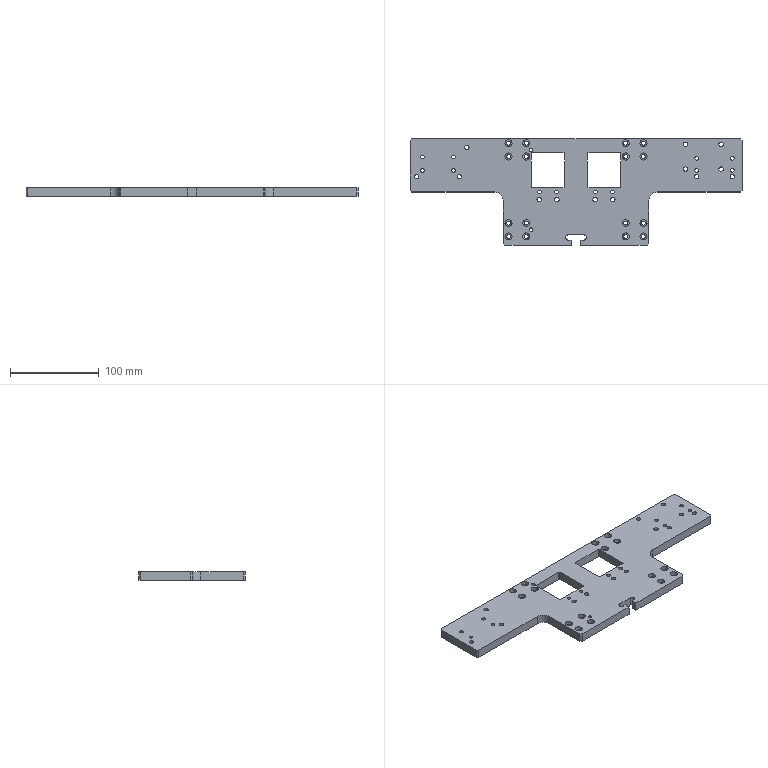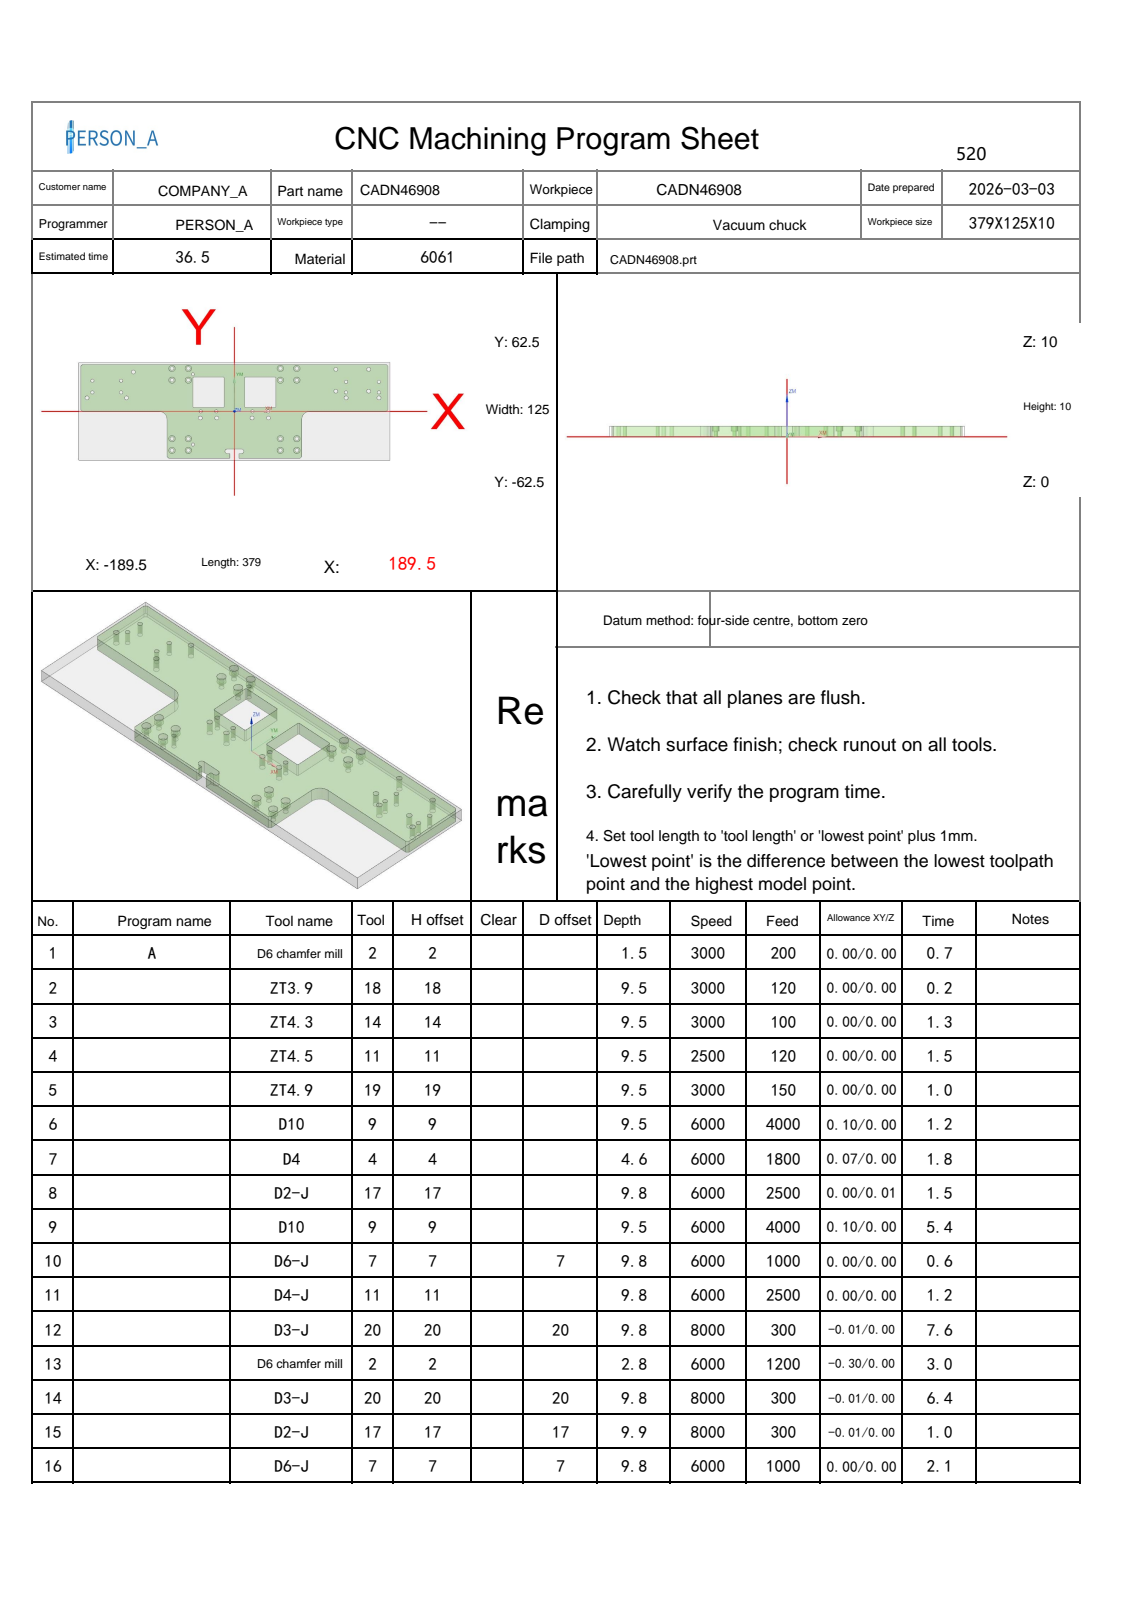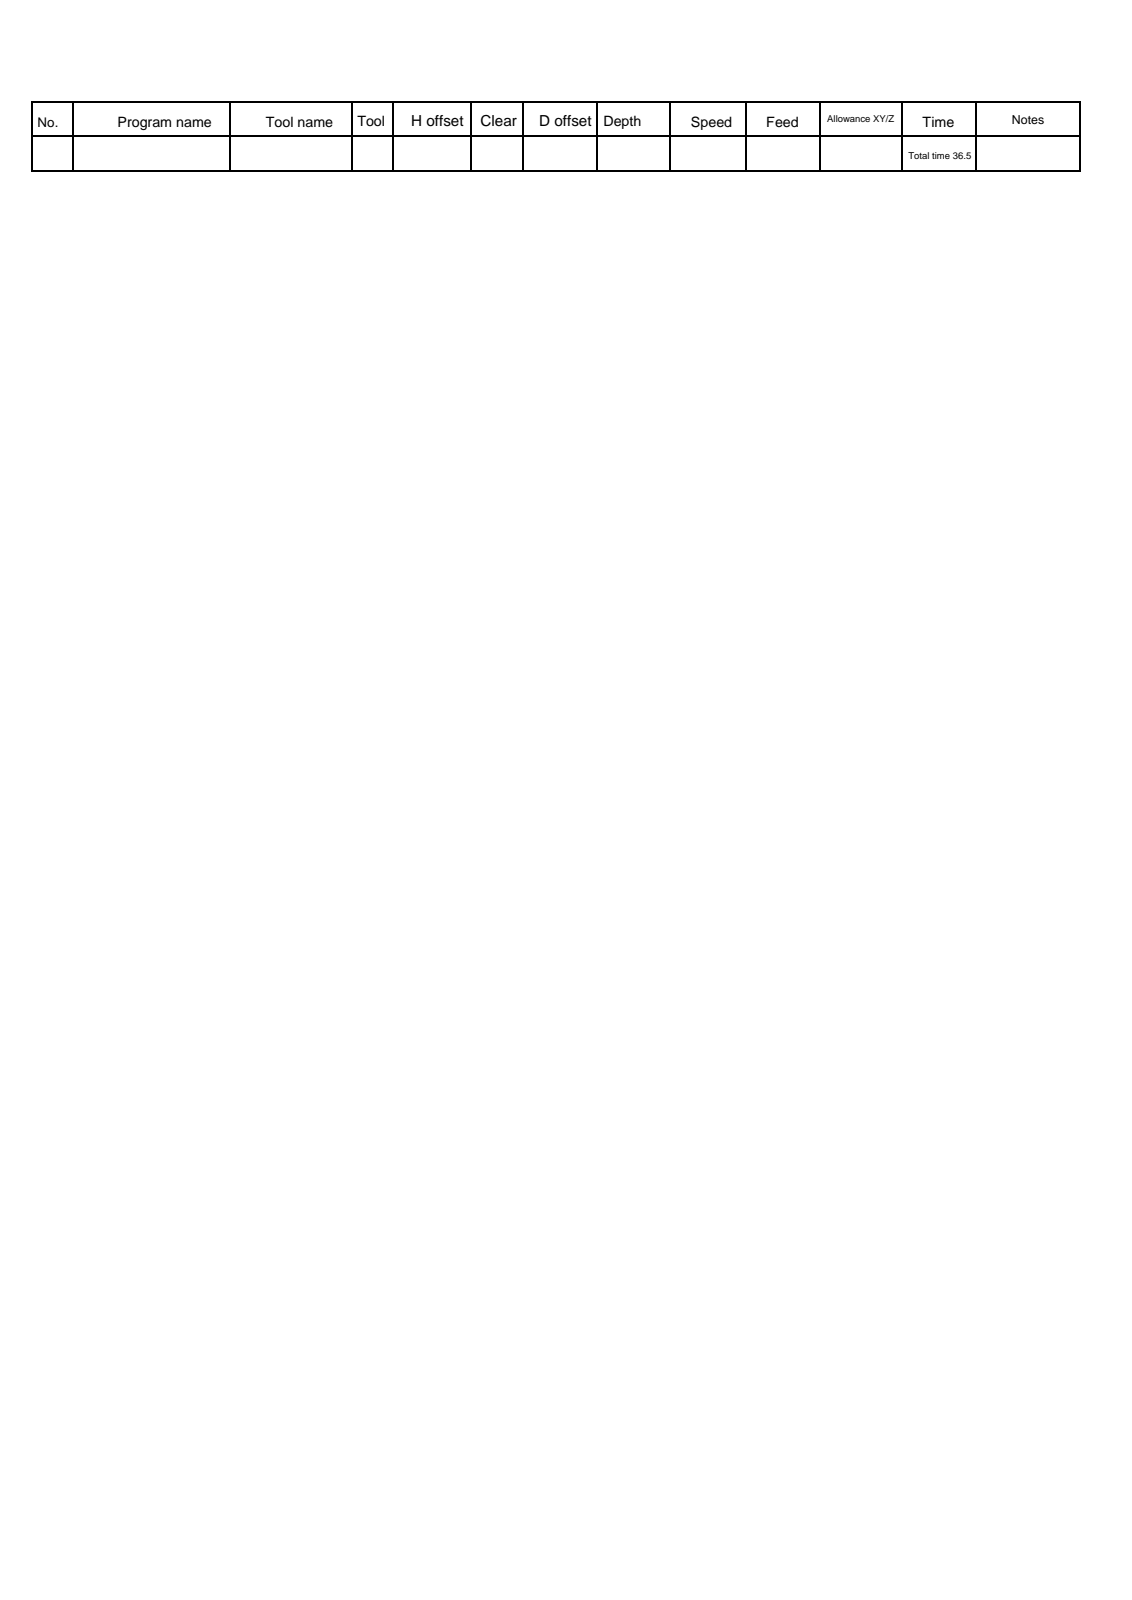NC program | NX | posted by the shop | part box 374 x 120 x 10 mm
Lines 1 to 769 of 15301:
%
O0001
(Machine time: 39.34 MIN)
(===Total Tool:10===)
(T2=D6 chamfer mill   D=6.   R=0.   D-  H02 Z=7.2   )
(T18=ZT3.9  D=3.9  DR_a=120 D-  H18 Z=0.5   )
(T14=ZT4.3  D=4.3  DR_a=118 D-  H14 Z=0.5   )
(T11=ZT4.5  D=4.5  DR_a=118 D-  H11 Z=0.2   )
(T19=ZT4.9  D=4.9  DR_a=120 D-  H19 Z=0.5   )
(T9=D10     D=10.  R=0.   D-  H09 Z=0.5   )
(T4=D4      D=4.   R=0.   D-  H04 Z=5.4   )
(T17=D2-J   D=2.   R=0.   D-  H17 Z=0.15  )
(T7=D6-J    D=6.   R=0.   D7  H07 Z=0.2   )
(T20=D3-J   D=3.   R=0.   D20 H20 Z=0.15  )
G80 G90 G17 G49 G40
G91 G28 Z0
M01
N1 T02 M06
(D6 chamfer mill  D=6. R=0. H=02 ce=0.00 di=0.00)
G00 G90 G54 X176. Y17.3 M03 S3000
G43 H02 Z40.
M08
G98 G82 X176. Y17.3 Z8.5 R11. F200.
X163.5 Y25.8
Y53.8
X123.5
Y25.8
X136. Y17.3
X41.5 Y-8.5
X21.5
X-21.5
X-41.5
X-122.971 Y50.4
X-131.471 Y17.3
X-179.471
G80
G00 Z40.
G00 G90 X-172.971 Y39.3 M03 S3000
Z40.
G98 G81 X-172.971 Y39.3 Z8.5 R11. F200.
Y24.3
X-137.971
Y39.3
X-76. Y40.
Y55.
X-56.
X-50.5 Y47.5
X-56. Y40.
X-76. Y-35.
Y-50.
X-56.
X-50.5 Y-42.5
X-56. Y-35.
X-41. Y0.0
X-22.
X22.
X41.
X56. Y-35.
Y-50.
X76.
Y-35.
X56. Y40.
Y55.
X76.
Y40.
X136. Y37.8
Y24.3
X176.
Y37.8
G80
G00 Z40.
G91 G28 Z0.0
M05
M09
G91 G28 Z0.0
M01
N2 T18 M06
(ZT3.9 D=3.9 DR_a=120 H=18)
G00 G90 G54 X-50.5 Y-42.5 M03 S3000
G43 H18 Z40.
M08
G98 G83 X-50.5 Y-42.5 Z.5 R11. F120. Q2.
Y47.5
G80
G00 Z40.
G91 G28 Z0.0
M05
M09
G91 G28 Z0.0
M01
N3 T14 M06
(ZT4.3 D=4.3 DR_a=118 H=14)
G00 G90 G54 X-172.971 Y24.3 M03 S3000
G43 H14 Z40.
M08
G98 G83 X-172.971 Y24.3 Z.5 R11. F100. Q1.5
Y39.3
X-137.971
Y24.3
X-41. Y0.0
X-22.
X22.
X41.
X136. Y24.3
Y37.8
X176.
Y24.3
G80
G00 Z40.
G91 G28 Z0.0
M05
M09
G91 G28 Z0.0
M01
N4 T11 M06
(ZT4.5 D=4.5 DR_a=118 H=11)
G00 G90 G54 X56. Y-35. M03 S2500
G43 H11 Z40.
M08
G98 G83 X56. Y-35. Z.5 R11. F120. Q3.
Y-50.
X76.
Y-35.
Y40.
Y55.
X56.
Y40.
X-56.
Y55.
X-76.
Y40.
Y-35.
Y-50.
X-56.
Y-35.
G80
G00 Z40.
G91 G28 Z0.0
M05
M09
G91 G28 Z0.0
M01
N5 T19 M06
(ZT4.9 D=4.9 DR_a=120 H=19)
G00 G90 G54 X176. Y17.3 M03 S3000
G43 H19 Z40.
M08
G98 G83 X176. Y17.3 Z.5 R11. F150. Q3.
X163.5 Y25.8
Y53.8
X123.5
Y25.8
X136. Y17.3
X41.5 Y-8.5
X21.5
X-21.5
X-41.5
X-122.971 Y50.4
X-131.471 Y17.3
X-179.471
G80
G00 Z40.
G91 G28 Z0.0
M05
M09
G91 G28 Z0.0
M01
N6 T09 M06
(D10  D=10. R=0. H=09 ce=0.10 di=0.00)
G00 G90 G54 X-31.5 Y38.9 M03 S6000
G43 H09 Z40.
M08
Z10.5
G01 X-45.4 Z10.439 F4000.
Y10.1 Z10.311
X-17.6 Z10.189
Y38.9 Z10.061
X-45.4 Z9.939
Y10.1 Z9.811
X-17.6 Z9.689
Y38.9 Z9.561
X-45.4 Z9.439
Y10.1 Z9.311
X-17.6 Z9.189
Y38.9 Z9.061
X-45.4 Z8.939
Y10.1 Z8.811
X-17.6 Z8.689
Y38.9 Z8.561
X-45.4 Z8.439
Y10.1 Z8.311
X-17.6 Z8.189
Y38.9 Z8.061
X-45.4 Z7.939
Y10.1 Z7.811
X-17.6 Z7.689
Y38.9 Z7.561
X-45.4 Z7.439
Y10.1 Z7.311
X-17.6 Z7.189
Y38.9 Z7.061
X-45.4 Z6.939
Y10.1 Z6.811
X-17.6 Z6.689
Y38.9 Z6.561
X-45.4 Z6.439
Y10.1 Z6.311
X-17.6 Z6.189
Y38.9 Z6.061
X-45.4 Z5.939
Y10.1 Z5.811
X-17.6 Z5.689
Y38.9 Z5.561
X-45.4 Z5.439
Y10.1 Z5.311
X-17.6 Z5.189
Y38.9 Z5.061
X-45.4 Z4.939
Y10.1 Z4.811
X-17.6 Z4.689
Y38.9 Z4.561
X-45.4 Z4.439
Y10.1 Z4.311
X-17.6 Z4.189
Y38.9 Z4.061
X-45.4 Z3.939
Y10.1 Z3.811
X-17.6 Z3.689
Y38.9 Z3.561
X-45.4 Z3.439
Y10.1 Z3.311
X-17.6 Z3.189
Y38.9 Z3.061
X-45.4 Z2.939
Y10.1 Z2.811
X-17.6 Z2.689
Y38.9 Z2.561
X-45.4 Z2.439
Y10.1 Z2.311
X-17.6 Z2.189
Y38.9 Z2.061
X-45.4 Z1.939
Y10.1 Z1.811
X-17.6 Z1.689
Y38.9 Z1.561
X-45.4 Z1.439
Y10.1 Z1.311
X-17.6 Z1.189
Y38.9 Z1.061
X-45.4 Z.939
Y10.1 Z.811
X-17.6 Z.689
Y38.9 Z.561
X-31.5 Z.5
X-45.4
Y10.1
X-17.6
Y38.9
X-31.5
X-32.
Z1.5
G00 Z40.
X31.5
Z10.5
G01 X17.6 Z10.439
Y10.1 Z10.311
X45.4 Z10.189
Y38.9 Z10.061
X17.6 Z9.939
Y10.1 Z9.811
X45.4 Z9.689
Y38.9 Z9.561
X17.6 Z9.439
Y10.1 Z9.311
X45.4 Z9.189
Y38.9 Z9.061
X17.6 Z8.939
Y10.1 Z8.811
X45.4 Z8.689
Y38.9 Z8.561
X17.6 Z8.439
Y10.1 Z8.311
X45.4 Z8.189
Y38.9 Z8.061
X17.6 Z7.939
Y10.1 Z7.811
X45.4 Z7.689
Y38.9 Z7.561
X17.6 Z7.439
Y10.1 Z7.311
X45.4 Z7.189
Y38.9 Z7.061
X17.6 Z6.939
Y10.1 Z6.811
X45.4 Z6.689
Y38.9 Z6.561
X17.6 Z6.439
Y10.1 Z6.311
X45.4 Z6.189
Y38.9 Z6.061
X17.6 Z5.939
Y10.1 Z5.811
X45.4 Z5.689
Y38.9 Z5.561
X17.6 Z5.439
Y10.1 Z5.311
X45.4 Z5.189
Y38.9 Z5.061
X17.6 Z4.939
Y10.1 Z4.811
X45.4 Z4.689
Y38.9 Z4.561
X17.6 Z4.439
Y10.1 Z4.311
X45.4 Z4.189
Y38.9 Z4.061
X17.6 Z3.939
Y10.1 Z3.811
X45.4 Z3.689
Y38.9 Z3.561
X17.6 Z3.439
Y10.1 Z3.311
X45.4 Z3.189
Y38.9 Z3.061
X17.6 Z2.939
Y10.1 Z2.811
X45.4 Z2.689
Y38.9 Z2.561
X17.6 Z2.439
Y10.1 Z2.311
X45.4 Z2.189
Y38.9 Z2.061
X17.6 Z1.939
Y10.1 Z1.811
X45.4 Z1.689
Y38.9 Z1.561
X17.6 Z1.439
Y10.1 Z1.311
X45.4 Z1.189
Y38.9 Z1.061
X17.6 Z.939
Y10.1 Z.811
X45.4 Z.689
Y38.9 Z.561
X31.5 Z.5
X17.6
Y10.1
X45.4
Y38.9
X31.5
X31.
Z1.5
G00 Z40.
G91 G28 Z0.0
M05
M09
G91 G28 Z0.0
M01
N7 T04 M06
(D4  D=4. R=0. H=04 ce=0.07 di=0.00)
G00 G90 G54 X-76. Y55. M03 S6000
G43 H04 Z40.
M08
Z10.3
G03 X-75.035 Y54.035 I.965 J0.0 F1800.
X-74.07 Y55. I0.0 J.965
X-74.07 Y55. Z9.95 I-1.93 J0.0
X-74.07 Y55. Z9.6 I-1.93 J0.0
X-74.07 Y55. Z9.25 I-1.93 J0.0
X-74.07 Y55. Z8.9 I-1.93 J0.0
X-74.07 Y55. Z8.55 I-1.93 J0.0
X-74.07 Y55. Z8.2 I-1.93 J0.0
X-74.07 Y55. Z7.85 I-1.93 J0.0
X-74.07 Y55. Z7.5 I-1.93 J0.0
X-74.07 Y55. Z7.15 I-1.93 J0.0
X-74.07 Y55. Z6.8 I-1.93 J0.0
X-74.07 Y55. Z6.45 I-1.93 J0.0
X-74.07 Y55. Z6.1 I-1.93 J0.0
X-74.07 Y55. Z5.75 I-1.93 J0.0
X-74.07 Y55. Z5.4 I-1.93 J0.0
X-76. Y56.93 I-1.93 J0.0
X-77.93 Y55. I0.0 J-1.93
X-76. Y53.07 I1.93 J0.0
X-74.07 Y55. I0.0 J1.93
X-75.035 Y55.965 I-.965 J0.0
X-76. Y55. I0.0 J-.965
G00 Z40.
X-56.
Z10.3
G03 X-55.035 Y54.035 I.965 J0.0
X-54.07 Y55. I0.0 J.965
X-54.07 Y55. Z9.95 I-1.93 J0.0
X-54.07 Y55. Z9.6 I-1.93 J0.0
X-54.07 Y55. Z9.25 I-1.93 J0.0
X-54.07 Y55. Z8.9 I-1.93 J0.0
X-54.07 Y55. Z8.55 I-1.93 J0.0
X-54.07 Y55. Z8.2 I-1.93 J0.0
X-54.07 Y55. Z7.85 I-1.93 J0.0
X-54.07 Y55. Z7.5 I-1.93 J0.0
X-54.07 Y55. Z7.15 I-1.93 J0.0
X-54.07 Y55. Z6.8 I-1.93 J0.0
X-54.07 Y55. Z6.45 I-1.93 J0.0
X-54.07 Y55. Z6.1 I-1.93 J0.0
X-54.07 Y55. Z5.75 I-1.93 J0.0
X-54.07 Y55. Z5.4 I-1.93 J0.0
X-56. Y56.93 I-1.93 J0.0
X-57.93 Y55. I0.0 J-1.93
X-56. Y53.07 I1.93 J0.0
X-54.07 Y55. I0.0 J1.93
X-55.035 Y55.965 I-.965 J0.0
X-56. Y55. I0.0 J-.965
G00 Z40.
Y40.
Z10.3
G03 X-55.035 Y39.035 I.965 J0.0
X-54.07 Y40. I0.0 J.965
X-54.07 Y40. Z9.95 I-1.93 J0.0
X-54.07 Y40. Z9.6 I-1.93 J0.0
X-54.07 Y40. Z9.25 I-1.93 J0.0
X-54.07 Y40. Z8.9 I-1.93 J0.0
X-54.07 Y40. Z8.55 I-1.93 J0.0
X-54.07 Y40. Z8.2 I-1.93 J0.0
X-54.07 Y40. Z7.85 I-1.93 J0.0
X-54.07 Y40. Z7.5 I-1.93 J0.0
X-54.07 Y40. Z7.15 I-1.93 J0.0
X-54.07 Y40. Z6.8 I-1.93 J0.0
X-54.07 Y40. Z6.45 I-1.93 J0.0
X-54.07 Y40. Z6.1 I-1.93 J0.0
X-54.07 Y40. Z5.75 I-1.93 J0.0
X-54.07 Y40. Z5.4 I-1.93 J0.0
X-56. Y41.93 I-1.93 J0.0
X-57.93 Y40. I0.0 J-1.93
X-56. Y38.07 I1.93 J0.0
X-54.07 Y40. I0.0 J1.93
X-55.035 Y40.965 I-.965 J0.0
X-56. Y40. I0.0 J-.965
G00 Z40.
X-76.
Z10.3
G03 X-75.035 Y39.035 I.965 J0.0
X-74.07 Y40. I0.0 J.965
X-74.07 Y40. Z9.95 I-1.93 J0.0
X-74.07 Y40. Z9.6 I-1.93 J0.0
X-74.07 Y40. Z9.25 I-1.93 J0.0
X-74.07 Y40. Z8.9 I-1.93 J0.0
X-74.07 Y40. Z8.55 I-1.93 J0.0
X-74.07 Y40. Z8.2 I-1.93 J0.0
X-74.07 Y40. Z7.85 I-1.93 J0.0
X-74.07 Y40. Z7.5 I-1.93 J0.0
X-74.07 Y40. Z7.15 I-1.93 J0.0
X-74.07 Y40. Z6.8 I-1.93 J0.0
X-74.07 Y40. Z6.45 I-1.93 J0.0
X-74.07 Y40. Z6.1 I-1.93 J0.0
X-74.07 Y40. Z5.75 I-1.93 J0.0
X-74.07 Y40. Z5.4 I-1.93 J0.0
X-76. Y41.93 I-1.93 J0.0
X-77.93 Y40. I0.0 J-1.93
X-76. Y38.07 I1.93 J0.0
X-74.07 Y40. I0.0 J1.93
X-75.035 Y40.965 I-.965 J0.0
X-76. Y40. I0.0 J-.965
G00 Z40.
Y-35.
Z10.3
G03 X-75.035 Y-35.965 I.965 J0.0
X-74.07 Y-35. I0.0 J.965
X-74.07 Y-35. Z9.95 I-1.93 J0.0
X-74.07 Y-35. Z9.6 I-1.93 J0.0
X-74.07 Y-35. Z9.25 I-1.93 J0.0
X-74.07 Y-35. Z8.9 I-1.93 J0.0
X-74.07 Y-35. Z8.55 I-1.93 J0.0
X-74.07 Y-35. Z8.2 I-1.93 J0.0
X-74.07 Y-35. Z7.85 I-1.93 J0.0
X-74.07 Y-35. Z7.5 I-1.93 J0.0
X-74.07 Y-35. Z7.15 I-1.93 J0.0
X-74.07 Y-35. Z6.8 I-1.93 J0.0
X-74.07 Y-35. Z6.45 I-1.93 J0.0
X-74.07 Y-35. Z6.1 I-1.93 J0.0
X-74.07 Y-35. Z5.75 I-1.93 J0.0
X-74.07 Y-35. Z5.4 I-1.93 J0.0
X-76. Y-33.07 I-1.93 J0.0
X-77.93 Y-35. I0.0 J-1.93
X-76. Y-36.93 I1.93 J0.0
X-74.07 Y-35. I0.0 J1.93
X-75.035 Y-34.035 I-.965 J0.0
X-76. Y-35. I0.0 J-.965
G00 Z40.
Y-50.
Z10.3
G03 X-75.035 Y-50.965 I.965 J0.0
X-74.07 Y-50. I0.0 J.965
X-74.07 Y-50. Z9.95 I-1.93 J0.0
X-74.07 Y-50. Z9.6 I-1.93 J0.0
X-74.07 Y-50. Z9.25 I-1.93 J0.0
X-74.07 Y-50. Z8.9 I-1.93 J0.0
X-74.07 Y-50. Z8.55 I-1.93 J0.0
X-74.07 Y-50. Z8.2 I-1.93 J0.0
X-74.07 Y-50. Z7.85 I-1.93 J0.0
X-74.07 Y-50. Z7.5 I-1.93 J0.0
X-74.07 Y-50. Z7.15 I-1.93 J0.0
X-74.07 Y-50. Z6.8 I-1.93 J0.0
X-74.07 Y-50. Z6.45 I-1.93 J0.0
X-74.07 Y-50. Z6.1 I-1.93 J0.0
X-74.07 Y-50. Z5.75 I-1.93 J0.0
X-74.07 Y-50. Z5.4 I-1.93 J0.0
X-76. Y-48.07 I-1.93 J0.0
X-77.93 Y-50. I0.0 J-1.93
X-76. Y-51.93 I1.93 J0.0
X-74.07 Y-50. I0.0 J1.93
X-75.035 Y-49.035 I-.965 J0.0
X-76. Y-50. I0.0 J-.965
G00 Z40.
X-56.
Z10.3
G03 X-55.035 Y-50.965 I.965 J0.0
X-54.07 Y-50. I0.0 J.965
X-54.07 Y-50. Z9.95 I-1.93 J0.0
X-54.07 Y-50. Z9.6 I-1.93 J0.0
X-54.07 Y-50. Z9.25 I-1.93 J0.0
X-54.07 Y-50. Z8.9 I-1.93 J0.0
X-54.07 Y-50. Z8.55 I-1.93 J0.0
X-54.07 Y-50. Z8.2 I-1.93 J0.0
X-54.07 Y-50. Z7.85 I-1.93 J0.0
X-54.07 Y-50. Z7.5 I-1.93 J0.0
X-54.07 Y-50. Z7.15 I-1.93 J0.0
X-54.07 Y-50. Z6.8 I-1.93 J0.0
X-54.07 Y-50. Z6.45 I-1.93 J0.0
X-54.07 Y-50. Z6.1 I-1.93 J0.0
X-54.07 Y-50. Z5.75 I-1.93 J0.0
X-54.07 Y-50. Z5.4 I-1.93 J0.0
X-56. Y-48.07 I-1.93 J0.0
X-57.93 Y-50. I0.0 J-1.93
X-56. Y-51.93 I1.93 J0.0
X-54.07 Y-50. I0.0 J1.93
X-55.035 Y-49.035 I-.965 J0.0
X-56. Y-50. I0.0 J-.965
G00 Z40.
Y-35.
Z10.3
G03 X-55.035 Y-35.965 I.965 J0.0
X-54.07 Y-35. I0.0 J.965
X-54.07 Y-35. Z9.95 I-1.93 J0.0
X-54.07 Y-35. Z9.6 I-1.93 J0.0
X-54.07 Y-35. Z9.25 I-1.93 J0.0
X-54.07 Y-35. Z8.9 I-1.93 J0.0
X-54.07 Y-35. Z8.55 I-1.93 J0.0
X-54.07 Y-35. Z8.2 I-1.93 J0.0
X-54.07 Y-35. Z7.85 I-1.93 J0.0
X-54.07 Y-35. Z7.5 I-1.93 J0.0
X-54.07 Y-35. Z7.15 I-1.93 J0.0
X-54.07 Y-35. Z6.8 I-1.93 J0.0
X-54.07 Y-35. Z6.45 I-1.93 J0.0
X-54.07 Y-35. Z6.1 I-1.93 J0.0
X-54.07 Y-35. Z5.75 I-1.93 J0.0
X-54.07 Y-35. Z5.4 I-1.93 J0.0
X-56. Y-33.07 I-1.93 J0.0
X-57.93 Y-35. I0.0 J-1.93
X-56. Y-36.93 I1.93 J0.0
X-54.07 Y-35. I0.0 J1.93
X-55.035 Y-34.035 I-.965 J0.0
X-56. Y-35. I0.0 J-.965
G00 Z40.
X56.
Z10.3
G03 X56.965 Y-35.965 I.965 J0.0
X57.93 Y-35. I0.0 J.965
X57.93 Y-35. Z9.95 I-1.93 J0.0
X57.93 Y-35. Z9.6 I-1.93 J0.0
X57.93 Y-35. Z9.25 I-1.93 J0.0
X57.93 Y-35. Z8.9 I-1.93 J0.0
X57.93 Y-35. Z8.55 I-1.93 J0.0
X57.93 Y-35. Z8.2 I-1.93 J0.0
X57.93 Y-35. Z7.85 I-1.93 J0.0
X57.93 Y-35. Z7.5 I-1.93 J0.0
X57.93 Y-35. Z7.15 I-1.93 J0.0
X57.93 Y-35. Z6.8 I-1.93 J0.0
X57.93 Y-35. Z6.45 I-1.93 J0.0
X57.93 Y-35. Z6.1 I-1.93 J0.0
X57.93 Y-35. Z5.75 I-1.93 J0.0
X57.93 Y-35. Z5.4 I-1.93 J0.0
X56. Y-33.07 I-1.93 J0.0
X54.07 Y-35. I0.0 J-1.93
X56. Y-36.93 I1.93 J0.0
X57.93 Y-35. I0.0 J1.93
X56.965 Y-34.035 I-.965 J0.0
X56. Y-35. I0.0 J-.965
G00 Z40.
Y-50.
Z10.3
G03 X56.965 Y-50.965 I.965 J0.0
X57.93 Y-50. I0.0 J.965
X57.93 Y-50. Z9.95 I-1.93 J0.0
X57.93 Y-50. Z9.6 I-1.93 J0.0
X57.93 Y-50. Z9.25 I-1.93 J0.0
X57.93 Y-50. Z8.9 I-1.93 J0.0
X57.93 Y-50. Z8.55 I-1.93 J0.0
X57.93 Y-50. Z8.2 I-1.93 J0.0
X57.93 Y-50. Z7.85 I-1.93 J0.0
X57.93 Y-50. Z7.5 I-1.93 J0.0
X57.93 Y-50. Z7.15 I-1.93 J0.0
X57.93 Y-50. Z6.8 I-1.93 J0.0
X57.93 Y-50. Z6.45 I-1.93 J0.0
X57.93 Y-50. Z6.1 I-1.93 J0.0
X57.93 Y-50. Z5.75 I-1.93 J0.0
X57.93 Y-50. Z5.4 I-1.93 J0.0
X56. Y-48.07 I-1.93 J0.0
X54.07 Y-50. I0.0 J-1.93
X56. Y-51.93 I1.93 J0.0
X57.93 Y-50. I0.0 J1.93
X56.965 Y-49.035 I-.965 J0.0
X56. Y-50. I0.0 J-.965
G00 Z40.
X76.
Z10.3
G03 X76.965 Y-50.965 I.965 J0.0
X77.93 Y-50. I0.0 J.965
X77.93 Y-50. Z9.95 I-1.93 J0.0
X77.93 Y-50. Z9.6 I-1.93 J0.0
X77.93 Y-50. Z9.25 I-1.93 J0.0
X77.93 Y-50. Z8.9 I-1.93 J0.0
X77.93 Y-50. Z8.55 I-1.93 J0.0
X77.93 Y-50. Z8.2 I-1.93 J0.0
X77.93 Y-50. Z7.85 I-1.93 J0.0
X77.93 Y-50. Z7.5 I-1.93 J0.0
X77.93 Y-50. Z7.15 I-1.93 J0.0
X77.93 Y-50. Z6.8 I-1.93 J0.0
X77.93 Y-50. Z6.45 I-1.93 J0.0
X77.93 Y-50. Z6.1 I-1.93 J0.0
X77.93 Y-50. Z5.75 I-1.93 J0.0
X77.93 Y-50. Z5.4 I-1.93 J0.0
X76. Y-48.07 I-1.93 J0.0
X74.07 Y-50. I0.0 J-1.93
X76. Y-51.93 I1.93 J0.0
X77.93 Y-50. I0.0 J1.93
X76.965 Y-49.035 I-.965 J0.0
X76. Y-50. I0.0 J-.965
G00 Z40.
Y-35.
Z10.3
G03 X76.965 Y-35.965 I.965 J0.0
X77.93 Y-35. I0.0 J.965
X77.93 Y-35. Z9.95 I-1.93 J0.0
X77.93 Y-35. Z9.6 I-1.93 J0.0
X77.93 Y-35. Z9.25 I-1.93 J0.0
X77.93 Y-35. Z8.9 I-1.93 J0.0
X77.93 Y-35. Z8.55 I-1.93 J0.0
X77.93 Y-35. Z8.2 I-1.93 J0.0
X77.93 Y-35. Z7.85 I-1.93 J0.0
X77.93 Y-35. Z7.5 I-1.93 J0.0
X77.93 Y-35. Z7.15 I-1.93 J0.0
X77.93 Y-35. Z6.8 I-1.93 J0.0
X77.93 Y-35. Z6.45 I-1.93 J0.0
X77.93 Y-35. Z6.1 I-1.93 J0.0
X77.93 Y-35. Z5.75 I-1.93 J0.0
X77.93 Y-35. Z5.4 I-1.93 J0.0
X76. Y-33.07 I-1.93 J0.0
X74.07 Y-35. I0.0 J-1.93
X76. Y-36.93 I1.93 J0.0
X77.93 Y-35. I0.0 J1.93
X76.965 Y-34.035 I-.965 J0.0
X76. Y-35. I0.0 J-.965
G00 Z40.
Y40.
Z10.3
G03 X76.965 Y39.035 I.965 J0.0
X77.93 Y40. I0.0 J.965
X77.93 Y40. Z9.95 I-1.93 J0.0
X77.93 Y40. Z9.6 I-1.93 J0.0
X77.93 Y40. Z9.25 I-1.93 J0.0
X77.93 Y40. Z8.9 I-1.93 J0.0
X77.93 Y40. Z8.55 I-1.93 J0.0
X77.93 Y40. Z8.2 I-1.93 J0.0
X77.93 Y40. Z7.85 I-1.93 J0.0
X77.93 Y40. Z7.5 I-1.93 J0.0
X77.93 Y40. Z7.15 I-1.93 J0.0
X77.93 Y40. Z6.8 I-1.93 J0.0
X77.93 Y40. Z6.45 I-1.93 J0.0
X77.93 Y40. Z6.1 I-1.93 J0.0
X77.93 Y40. Z5.75 I-1.93 J0.0
X77.93 Y40. Z5.4 I-1.93 J0.0
X76. Y41.93 I-1.93 J0.0
X74.07 Y40. I0.0 J-1.93
X76. Y38.07 I1.93 J0.0
X77.93 Y40. I0.0 J1.93
X76.965 Y40.965 I-.965 J0.0
X76. Y40. I0.0 J-.965
G00 Z40.
Y55.
Z10.3
G03 X76.965 Y54.035 I.965 J0.0
X77.93 Y55. I0.0 J.965
X77.93 Y55. Z9.95 I-1.93 J0.0
X77.93 Y55. Z9.6 I-1.93 J0.0
X77.93 Y55. Z9.25 I-1.93 J0.0
X77.93 Y55. Z8.9 I-1.93 J0.0
X77.93 Y55. Z8.55 I-1.93 J0.0
X77.93 Y55. Z8.2 I-1.93 J0.0
X77.93 Y55. Z7.85 I-1.93 J0.0
X77.93 Y55. Z7.5 I-1.93 J0.0
X77.93 Y55. Z7.15 I-1.93 J0.0
X77.93 Y55. Z6.8 I-1.93 J0.0
X77.93 Y55. Z6.45 I-1.93 J0.0
X77.93 Y55. Z6.1 I-1.93 J0.0
X77.93 Y55. Z5.75 I-1.93 J0.0
X77.93 Y55. Z5.4 I-1.93 J0.0
X76. Y56.93 I-1.93 J0.0
X74.07 Y55. I0.0 J-1.93
X76. Y53.07 I1.93 J0.0
X77.93 Y55. I0.0 J1.93
X76.965 Y55.965 I-.965 J0.0
X76. Y55. I0.0 J-.965
G00 Z40.
X56.
Z10.3
G03 X56.965 Y54.035 I.965 J0.0
X57.93 Y55. I0.0 J.965
X57.93 Y55. Z9.95 I-1.93 J0.0
X57.93 Y55. Z9.6 I-1.93 J0.0
X57.93 Y55. Z9.25 I-1.93 J0.0
X57.93 Y55. Z8.9 I-1.93 J0.0
X57.93 Y55. Z8.55 I-1.93 J0.0
X57.93 Y55. Z8.2 I-1.93 J0.0
X57.93 Y55. Z7.85 I-1.93 J0.0
X57.93 Y55. Z7.5 I-1.93 J0.0
X57.93 Y55. Z7.15 I-1.93 J0.0
X57.93 Y55. Z6.8 I-1.93 J0.0
X57.93 Y55. Z6.45 I-1.93 J0.0
X57.93 Y55. Z6.1 I-1.93 J0.0
X57.93 Y55. Z5.75 I-1.93 J0.0
X57.93 Y55. Z5.4 I-1.93 J0.0
X56. Y56.93 I-1.93 J0.0
X54.07 Y55. I0.0 J-1.93
X56. Y53.07 I1.93 J0.0
X57.93 Y55. I0.0 J1.93
X56.965 Y55.965 I-.965 J0.0
X56. Y55. I0.0 J-.965
G00 Z40.
Y40.
Z10.3
G03 X56.965 Y39.035 I.965 J0.0
X57.93 Y40. I0.0 J.965
X57.93 Y40. Z9.95 I-1.93 J0.0
X57.93 Y40. Z9.6 I-1.93 J0.0
X57.93 Y40. Z9.25 I-1.93 J0.0
X57.93 Y40. Z8.9 I-1.93 J0.0
X57.93 Y40. Z8.55 I-1.93 J0.0
X57.93 Y40. Z8.2 I-1.93 J0.0
X57.93 Y40. Z7.85 I-1.93 J0.0
X57.93 Y40. Z7.5 I-1.93 J0.0
X57.93 Y40. Z7.15 I-1.93 J0.0
X57.93 Y40. Z6.8 I-1.93 J0.0
X57.93 Y40. Z6.45 I-1.93 J0.0
X57.93 Y40. Z6.1 I-1.93 J0.0
X57.93 Y40. Z5.75 I-1.93 J0.0
X57.93 Y40. Z5.4 I-1.93 J0.0
X56. Y41.93 I-1.93 J0.0
X54.07 Y40. I0.0 J-1.93
X56. Y38.07 I1.93 J0.0
X57.93 Y40. I0.0 J1.93
X56.965 Y40.965 I-.965 J0.0
X56. Y40. I0.0 J-.965
G00 Z40.
G91 G28 Z0.0
M05
M09
G91 G28 Z0.0
M01